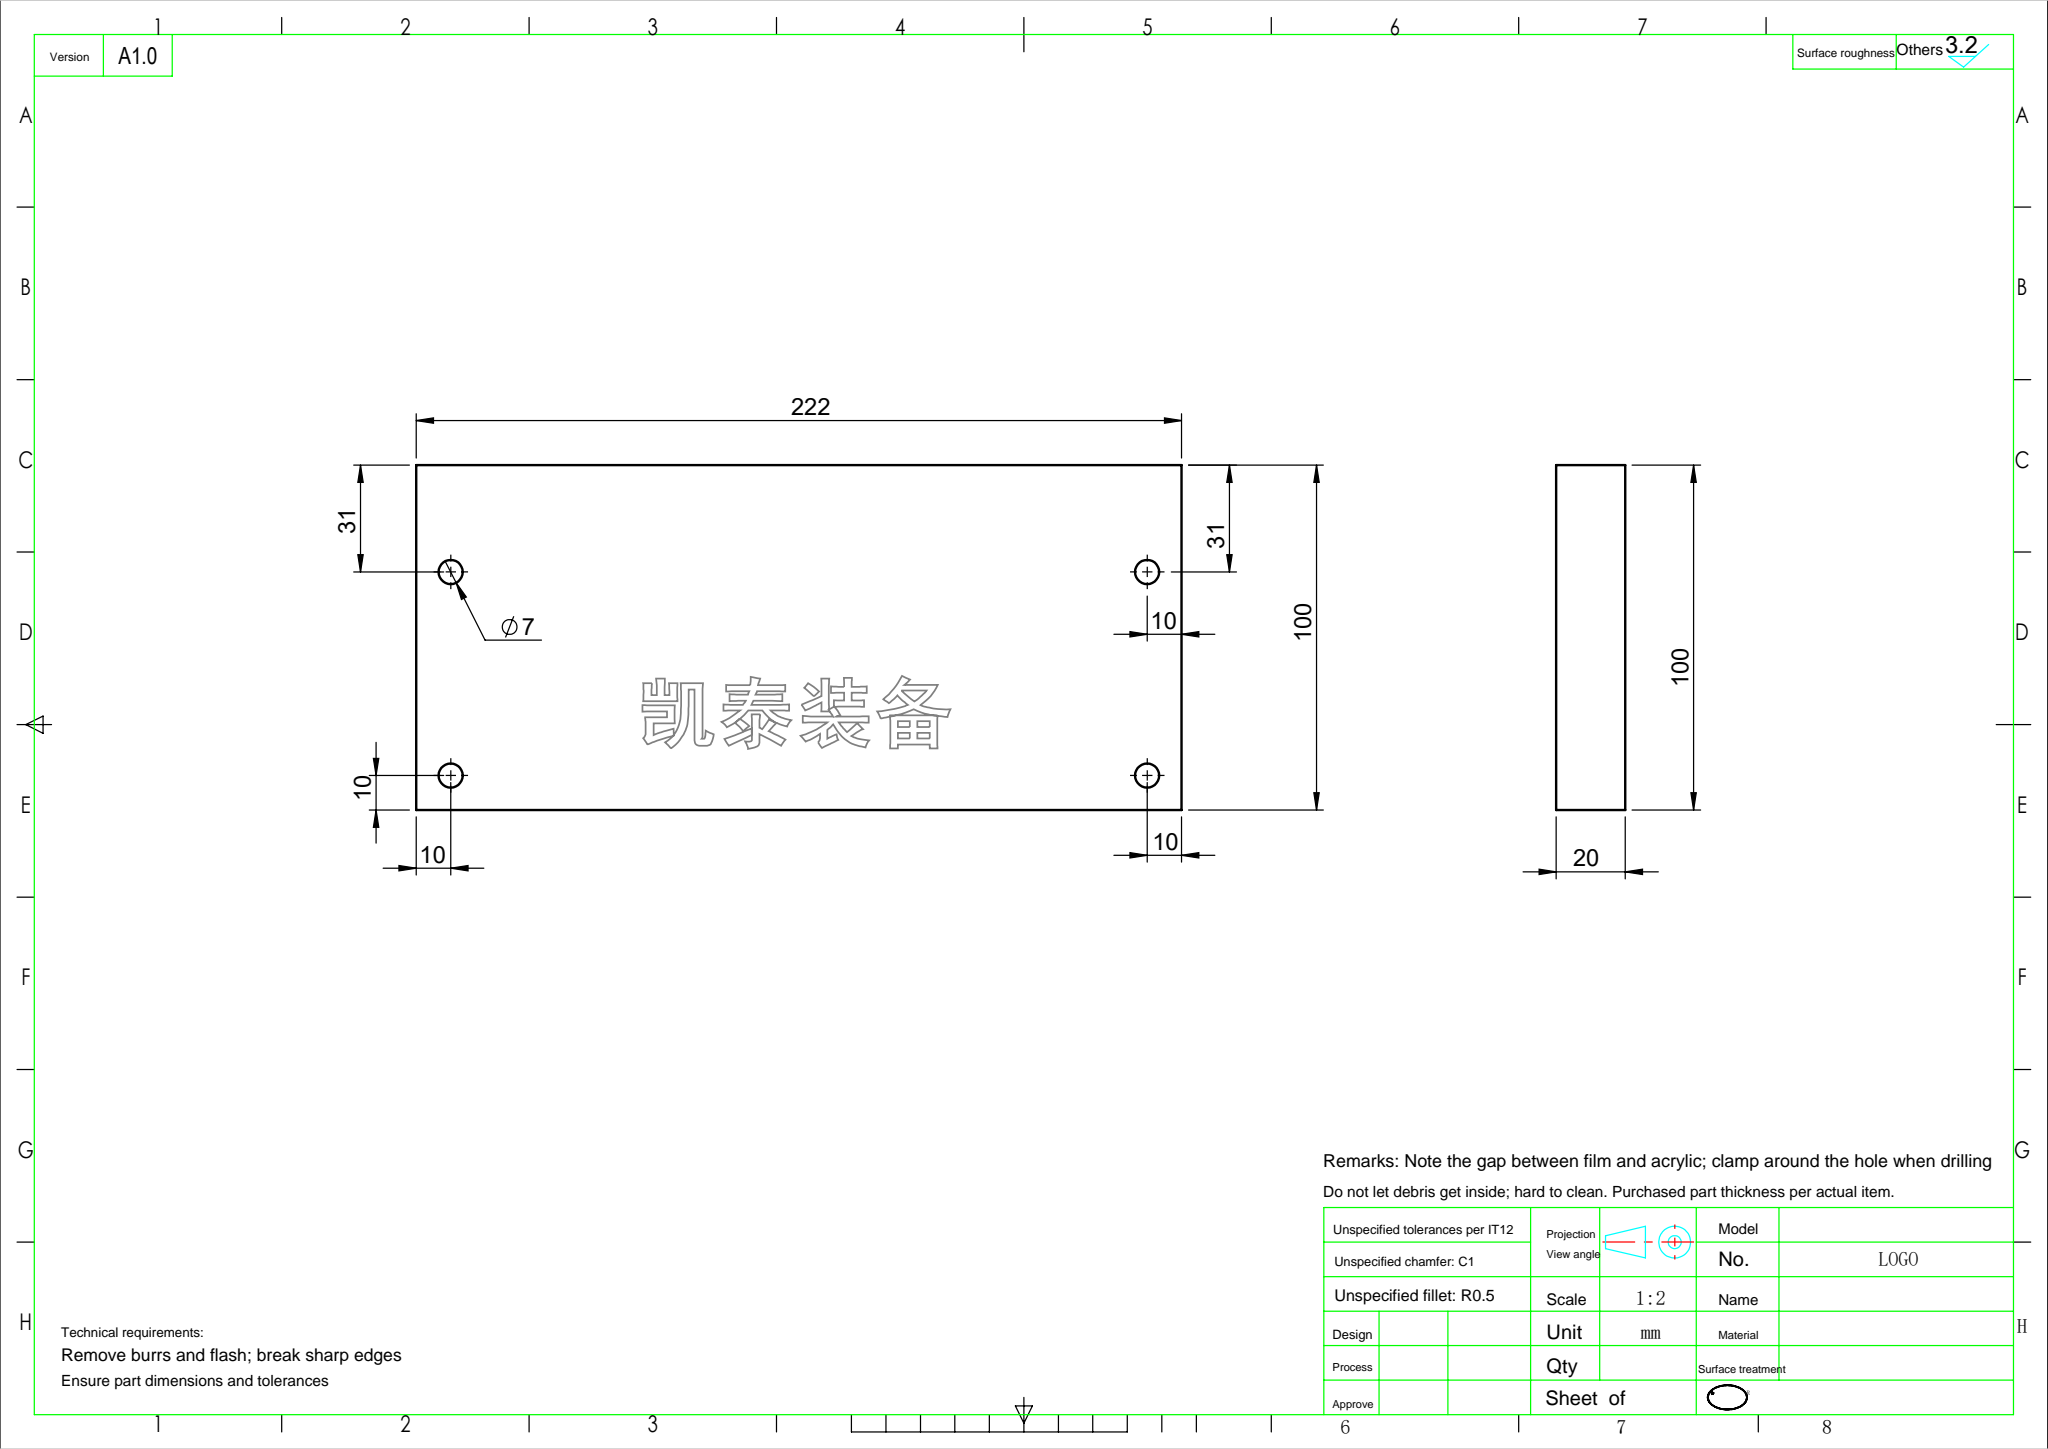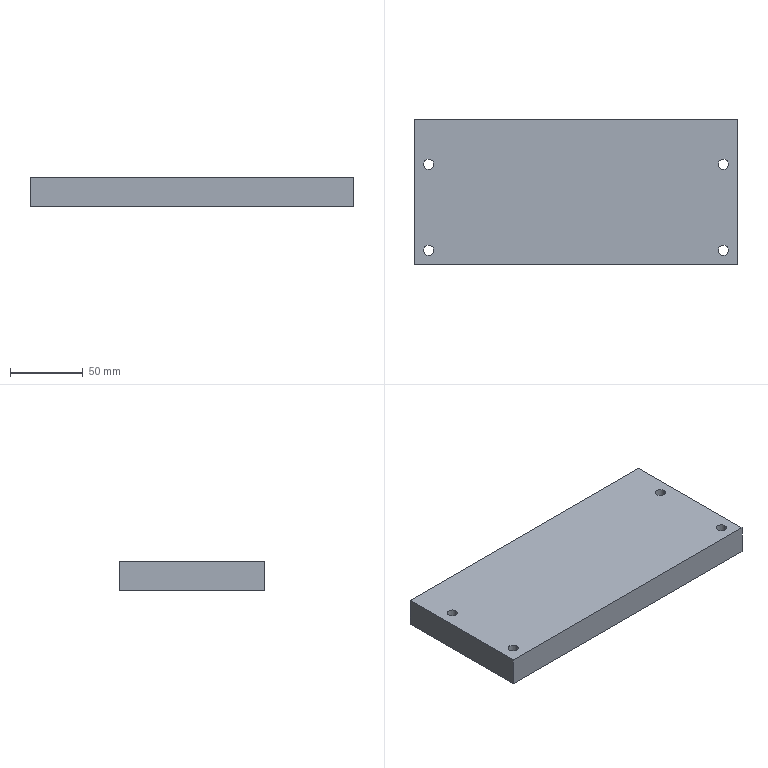Part | SolidWorks | features Extrusion 1, ICE 1 | 1 solid | 14 faces | box 222 x 100 x 20 mm | volume 440921 mm3 | cylinder 8 | plane 6 | commonest cylinder face diameters 7 x8
STEP:
#1=CARTESIAN_POINT('',(-104.5,-40.,0.));
#2=VERTEX_POINT('',#1);
#3=CARTESIAN_POINT('',(-97.5,-40.,0.));
#4=VERTEX_POINT('',#3);
#5=CARTESIAN_POINT('',(-101.,-40.,0.));
#6=DIRECTION('',(0.,0.,1.));
#7=DIRECTION('',(1.,0.,0.));
#8=AXIS2_PLACEMENT_3D('',#5,#6,#7);
#9=CIRCLE('',#8,3.5);
#10=EDGE_CURVE('',#2,#4,#9,.T.);
#11=ORIENTED_EDGE('',*,*,#10,.F.);
#12=CARTESIAN_POINT('',(-104.5,-40.,20.));
#13=VERTEX_POINT('',#12);
#14=CARTESIAN_POINT('',(-104.5,-40.,0.));
#15=DIRECTION('',(0.,0.,1.));
#16=VECTOR('',#15,1000.);
#17=LINE('',#14,#16);
#18=EDGE_CURVE('',#2,#13,#17,.T.);
#19=ORIENTED_EDGE('',*,*,#18,.T.);
#20=CARTESIAN_POINT('',(-97.5,-40.,20.));
#21=VERTEX_POINT('',#20);
#22=CARTESIAN_POINT('',(-101.,-40.,20.));
#23=DIRECTION('',(0.,0.,1.));
#24=DIRECTION('',(1.,0.,0.));
#25=AXIS2_PLACEMENT_3D('',#22,#23,#24);
#26=CIRCLE('',#25,3.5);
#27=EDGE_CURVE('',#13,#21,#26,.T.);
#28=ORIENTED_EDGE('',*,*,#27,.T.);
#29=CARTESIAN_POINT('',(-97.5,-40.,0.));
#30=DIRECTION('',(0.,0.,1.));
#31=VECTOR('',#30,1000.);
#32=LINE('',#29,#31);
#33=EDGE_CURVE('',#4,#21,#32,.T.);
#34=ORIENTED_EDGE('',*,*,#33,.F.);
#35=EDGE_LOOP('',(#11,#19,#28,#34));
#36=FACE_OUTER_BOUND('',#35,.T.);
#37=CARTESIAN_POINT('',(-101.,-40.,0.));
#38=DIRECTION('',(0.,0.,1.));
#39=DIRECTION('',(1.,0.,0.));
#40=AXIS2_PLACEMENT_3D('',#37,#38,#39);
#41=CYLINDRICAL_SURFACE('',#40,3.5);
#42=ADVANCED_FACE('',(#36),#41,.F.);
#43=CARTESIAN_POINT('',(97.5,19.,0.));
#44=VERTEX_POINT('',#43);
#45=CARTESIAN_POINT('',(104.5,19.,0.));
#46=VERTEX_POINT('',#45);
#47=CARTESIAN_POINT('',(101.,19.,0.));
#48=DIRECTION('',(0.,0.,1.));
#49=DIRECTION('',(1.,0.,0.));
#50=AXIS2_PLACEMENT_3D('',#47,#48,#49);
#51=CIRCLE('',#50,3.5);
#52=EDGE_CURVE('',#44,#46,#51,.T.);
#53=ORIENTED_EDGE('',*,*,#52,.F.);
#54=CARTESIAN_POINT('',(97.5,19.,20.));
#55=VERTEX_POINT('',#54);
#56=CARTESIAN_POINT('',(97.5,19.,0.));
#57=DIRECTION('',(0.,0.,1.));
#58=VECTOR('',#57,1000.);
#59=LINE('',#56,#58);
#60=EDGE_CURVE('',#44,#55,#59,.T.);
#61=ORIENTED_EDGE('',*,*,#60,.T.);
#62=CARTESIAN_POINT('',(104.5,19.,20.));
#63=VERTEX_POINT('',#62);
#64=CARTESIAN_POINT('',(101.,19.,20.));
#65=DIRECTION('',(0.,0.,1.));
#66=DIRECTION('',(1.,0.,0.));
#67=AXIS2_PLACEMENT_3D('',#64,#65,#66);
#68=CIRCLE('',#67,3.5);
#69=EDGE_CURVE('',#55,#63,#68,.T.);
#70=ORIENTED_EDGE('',*,*,#69,.T.);
#71=CARTESIAN_POINT('',(104.5,19.,0.));
#72=DIRECTION('',(0.,0.,1.));
#73=VECTOR('',#72,1000.);
#74=LINE('',#71,#73);
#75=EDGE_CURVE('',#46,#63,#74,.T.);
#76=ORIENTED_EDGE('',*,*,#75,.F.);
#77=EDGE_LOOP('',(#53,#61,#70,#76));
#78=FACE_OUTER_BOUND('',#77,.T.);
#79=CARTESIAN_POINT('',(101.,19.,0.));
#80=DIRECTION('',(0.,0.,1.));
#81=DIRECTION('',(1.,0.,0.));
#82=AXIS2_PLACEMENT_3D('',#79,#80,#81);
#83=CYLINDRICAL_SURFACE('',#82,3.5);
#84=ADVANCED_FACE('',(#78),#83,.F.);
#85=CARTESIAN_POINT('',(97.5,-40.,0.));
#86=VERTEX_POINT('',#85);
#87=CARTESIAN_POINT('',(104.5,-40.,0.));
#88=VERTEX_POINT('',#87);
#89=CARTESIAN_POINT('',(101.,-40.,0.));
#90=DIRECTION('',(0.,0.,1.));
#91=DIRECTION('',(1.,0.,0.));
#92=AXIS2_PLACEMENT_3D('',#89,#90,#91);
#93=CIRCLE('',#92,3.5);
#94=EDGE_CURVE('',#86,#88,#93,.T.);
#95=ORIENTED_EDGE('',*,*,#94,.F.);
#96=CARTESIAN_POINT('',(97.5,-40.,20.));
#97=VERTEX_POINT('',#96);
#98=CARTESIAN_POINT('',(97.5,-40.,0.));
#99=DIRECTION('',(0.,0.,1.));
#100=VECTOR('',#99,1000.);
#101=LINE('',#98,#100);
#102=EDGE_CURVE('',#86,#97,#101,.T.);
#103=ORIENTED_EDGE('',*,*,#102,.T.);
#104=CARTESIAN_POINT('',(104.5,-40.,20.));
#105=VERTEX_POINT('',#104);
#106=CARTESIAN_POINT('',(101.,-40.,20.));
#107=DIRECTION('',(0.,0.,1.));
#108=DIRECTION('',(1.,0.,0.));
#109=AXIS2_PLACEMENT_3D('',#106,#107,#108);
#110=CIRCLE('',#109,3.5);
#111=EDGE_CURVE('',#97,#105,#110,.T.);
#112=ORIENTED_EDGE('',*,*,#111,.T.);
#113=CARTESIAN_POINT('',(104.5,-40.,0.));
#114=DIRECTION('',(0.,0.,1.));
#115=VECTOR('',#114,1000.);
#116=LINE('',#113,#115);
#117=EDGE_CURVE('',#88,#105,#116,.T.);
#118=ORIENTED_EDGE('',*,*,#117,.F.);
#119=EDGE_LOOP('',(#95,#103,#112,#118));
#120=FACE_OUTER_BOUND('',#119,.T.);
#121=CARTESIAN_POINT('',(101.,-40.,0.));
#122=DIRECTION('',(0.,0.,1.));
#123=DIRECTION('',(1.,0.,0.));
#124=AXIS2_PLACEMENT_3D('',#121,#122,#123);
#125=CYLINDRICAL_SURFACE('',#124,3.5);
#126=ADVANCED_FACE('',(#120),#125,.F.);
#127=CARTESIAN_POINT('',(-104.5,19.,0.));
#128=VERTEX_POINT('',#127);
#129=CARTESIAN_POINT('',(-97.5,19.,0.));
#130=VERTEX_POINT('',#129);
#131=CARTESIAN_POINT('',(-101.,19.,0.));
#132=DIRECTION('',(0.,0.,1.));
#133=DIRECTION('',(1.,0.,0.));
#134=AXIS2_PLACEMENT_3D('',#131,#132,#133);
#135=CIRCLE('',#134,3.5);
#136=EDGE_CURVE('',#128,#130,#135,.T.);
#137=ORIENTED_EDGE('',*,*,#136,.F.);
#138=CARTESIAN_POINT('',(-104.5,19.,20.));
#139=VERTEX_POINT('',#138);
#140=CARTESIAN_POINT('',(-104.5,19.,0.));
#141=DIRECTION('',(0.,0.,1.));
#142=VECTOR('',#141,1000.);
#143=LINE('',#140,#142);
#144=EDGE_CURVE('',#128,#139,#143,.T.);
#145=ORIENTED_EDGE('',*,*,#144,.T.);
#146=CARTESIAN_POINT('',(-97.5,19.,20.));
#147=VERTEX_POINT('',#146);
#148=CARTESIAN_POINT('',(-101.,19.,20.));
#149=DIRECTION('',(0.,0.,1.));
#150=DIRECTION('',(1.,0.,0.));
#151=AXIS2_PLACEMENT_3D('',#148,#149,#150);
#152=CIRCLE('',#151,3.5);
#153=EDGE_CURVE('',#139,#147,#152,.T.);
#154=ORIENTED_EDGE('',*,*,#153,.T.);
#155=CARTESIAN_POINT('',(-97.5,19.,0.));
#156=DIRECTION('',(0.,0.,1.));
#157=VECTOR('',#156,1000.);
#158=LINE('',#155,#157);
#159=EDGE_CURVE('',#130,#147,#158,.T.);
#160=ORIENTED_EDGE('',*,*,#159,.F.);
#161=EDGE_LOOP('',(#137,#145,#154,#160));
#162=FACE_OUTER_BOUND('',#161,.T.);
#163=CARTESIAN_POINT('',(-101.,19.,0.));
#164=DIRECTION('',(0.,0.,1.));
#165=DIRECTION('',(1.,0.,0.));
#166=AXIS2_PLACEMENT_3D('',#163,#164,#165);
#167=CYLINDRICAL_SURFACE('',#166,3.5);
#168=ADVANCED_FACE('',(#162),#167,.F.);
#169=CARTESIAN_POINT('',(111.,-50.,0.));
#170=VERTEX_POINT('',#169);
#171=CARTESIAN_POINT('',(111.,50.,0.));
#172=VERTEX_POINT('',#171);
#173=CARTESIAN_POINT('',(111.,50.,0.));
#174=DIRECTION('',(0.,1.,0.));
#175=VECTOR('',#174,1000.);
#176=LINE('',#173,#175);
#177=EDGE_CURVE('',#170,#172,#176,.T.);
#178=ORIENTED_EDGE('',*,*,#177,.T.);
#179=CARTESIAN_POINT('',(111.,50.,20.));
#180=VERTEX_POINT('',#179);
#181=CARTESIAN_POINT('',(111.,50.,20.));
#182=DIRECTION('',(0.,0.,-1.));
#183=VECTOR('',#182,1000.);
#184=LINE('',#181,#183);
#185=EDGE_CURVE('',#180,#172,#184,.T.);
#186=ORIENTED_EDGE('',*,*,#185,.F.);
#187=CARTESIAN_POINT('',(111.,-50.,20.));
#188=VERTEX_POINT('',#187);
#189=CARTESIAN_POINT('',(111.,50.,20.));
#190=DIRECTION('',(0.,1.,0.));
#191=VECTOR('',#190,1000.);
#192=LINE('',#189,#191);
#193=EDGE_CURVE('',#188,#180,#192,.T.);
#194=ORIENTED_EDGE('',*,*,#193,.F.);
#195=CARTESIAN_POINT('',(111.,-50.,20.));
#196=DIRECTION('',(0.,0.,-1.));
#197=VECTOR('',#196,1000.);
#198=LINE('',#195,#197);
#199=EDGE_CURVE('',#188,#170,#198,.T.);
#200=ORIENTED_EDGE('',*,*,#199,.T.);
#201=EDGE_LOOP('',(#178,#186,#194,#200));
#202=FACE_OUTER_BOUND('',#201,.T.);
#203=CARTESIAN_POINT('',(111.,50.,20.));
#204=DIRECTION('',(-1.,0.,0.));
#205=DIRECTION('',(0.,-1.,0.));
#206=AXIS2_PLACEMENT_3D('',#203,#204,#205);
#207=PLANE('',#206);
#208=ADVANCED_FACE('',(#202),#207,.F.);
#209=CARTESIAN_POINT('',(-111.,50.,0.));
#210=VERTEX_POINT('',#209);
#211=CARTESIAN_POINT('',(-111.,50.,0.));
#212=DIRECTION('',(-1.,0.,0.));
#213=VECTOR('',#212,1000.);
#214=LINE('',#211,#213);
#215=EDGE_CURVE('',#172,#210,#214,.T.);
#216=ORIENTED_EDGE('',*,*,#215,.T.);
#217=CARTESIAN_POINT('',(-111.,50.,20.));
#218=VERTEX_POINT('',#217);
#219=CARTESIAN_POINT('',(-111.,50.,20.));
#220=DIRECTION('',(0.,0.,-1.));
#221=VECTOR('',#220,1000.);
#222=LINE('',#219,#221);
#223=EDGE_CURVE('',#218,#210,#222,.T.);
#224=ORIENTED_EDGE('',*,*,#223,.F.);
#225=CARTESIAN_POINT('',(-111.,50.,20.));
#226=DIRECTION('',(-1.,0.,0.));
#227=VECTOR('',#226,1000.);
#228=LINE('',#225,#227);
#229=EDGE_CURVE('',#180,#218,#228,.T.);
#230=ORIENTED_EDGE('',*,*,#229,.F.);
#231=ORIENTED_EDGE('',*,*,#185,.T.);
#232=EDGE_LOOP('',(#216,#224,#230,#231));
#233=FACE_OUTER_BOUND('',#232,.T.);
#234=CARTESIAN_POINT('',(-111.,50.,20.));
#235=DIRECTION('',(0.,-1.,0.));
#236=DIRECTION('',(0.,0.,-1.));
#237=AXIS2_PLACEMENT_3D('',#234,#235,#236);
#238=PLANE('',#237);
#239=ADVANCED_FACE('',(#233),#238,.F.);
#240=CARTESIAN_POINT('',(-111.,-50.,0.));
#241=VERTEX_POINT('',#240);
#242=CARTESIAN_POINT('',(-111.,50.,0.));
#243=DIRECTION('',(0.,-1.,0.));
#244=VECTOR('',#243,1000.);
#245=LINE('',#242,#244);
#246=EDGE_CURVE('',#210,#241,#245,.T.);
#247=ORIENTED_EDGE('',*,*,#246,.T.);
#248=CARTESIAN_POINT('',(-111.,-50.,20.));
#249=VERTEX_POINT('',#248);
#250=CARTESIAN_POINT('',(-111.,-50.,20.));
#251=DIRECTION('',(0.,0.,-1.));
#252=VECTOR('',#251,1000.);
#253=LINE('',#250,#252);
#254=EDGE_CURVE('',#249,#241,#253,.T.);
#255=ORIENTED_EDGE('',*,*,#254,.F.);
#256=CARTESIAN_POINT('',(-111.,50.,20.));
#257=DIRECTION('',(0.,-1.,0.));
#258=VECTOR('',#257,1000.);
#259=LINE('',#256,#258);
#260=EDGE_CURVE('',#218,#249,#259,.T.);
#261=ORIENTED_EDGE('',*,*,#260,.F.);
#262=ORIENTED_EDGE('',*,*,#223,.T.);
#263=EDGE_LOOP('',(#247,#255,#261,#262));
#264=FACE_OUTER_BOUND('',#263,.T.);
#265=CARTESIAN_POINT('',(-111.,50.,20.));
#266=DIRECTION('',(1.,0.,0.));
#267=DIRECTION('',(0.,1.,0.));
#268=AXIS2_PLACEMENT_3D('',#265,#266,#267);
#269=PLANE('',#268);
#270=ADVANCED_FACE('',(#264),#269,.F.);
#271=CARTESIAN_POINT('',(-111.,-50.,0.));
#272=DIRECTION('',(1.,0.,0.));
#273=VECTOR('',#272,1000.);
#274=LINE('',#271,#273);
#275=EDGE_CURVE('',#241,#170,#274,.T.);
#276=ORIENTED_EDGE('',*,*,#275,.T.);
#277=ORIENTED_EDGE('',*,*,#199,.F.);
#278=CARTESIAN_POINT('',(-111.,-50.,20.));
#279=DIRECTION('',(1.,0.,0.));
#280=VECTOR('',#279,1000.);
#281=LINE('',#278,#280);
#282=EDGE_CURVE('',#249,#188,#281,.T.);
#283=ORIENTED_EDGE('',*,*,#282,.F.);
#284=ORIENTED_EDGE('',*,*,#254,.T.);
#285=EDGE_LOOP('',(#276,#277,#283,#284));
#286=FACE_OUTER_BOUND('',#285,.T.);
#287=CARTESIAN_POINT('',(-111.,-50.,20.));
#288=DIRECTION('',(0.,1.,0.));
#289=DIRECTION('',(0.,0.,1.));
#290=AXIS2_PLACEMENT_3D('',#287,#288,#289);
#291=PLANE('',#290);
#292=ADVANCED_FACE('',(#286),#291,.F.);
#293=CARTESIAN_POINT('',(-101.,-40.,20.));
#294=DIRECTION('',(0.,0.,1.));
#295=DIRECTION('',(1.,0.,0.));
#296=AXIS2_PLACEMENT_3D('',#293,#294,#295);
#297=CIRCLE('',#296,3.5);
#298=EDGE_CURVE('',#21,#13,#297,.T.);
#299=ORIENTED_EDGE('',*,*,#298,.F.);
#300=ORIENTED_EDGE('',*,*,#27,.F.);
#301=EDGE_LOOP('',(#299,#300));
#302=FACE_BOUND('',#301,.T.);
#303=CARTESIAN_POINT('',(101.,19.,20.));
#304=DIRECTION('',(0.,0.,1.));
#305=DIRECTION('',(1.,0.,0.));
#306=AXIS2_PLACEMENT_3D('',#303,#304,#305);
#307=CIRCLE('',#306,3.5);
#308=EDGE_CURVE('',#63,#55,#307,.T.);
#309=ORIENTED_EDGE('',*,*,#308,.F.);
#310=ORIENTED_EDGE('',*,*,#69,.F.);
#311=EDGE_LOOP('',(#309,#310));
#312=FACE_BOUND('',#311,.T.);
#313=CARTESIAN_POINT('',(101.,-40.,20.));
#314=DIRECTION('',(0.,0.,1.));
#315=DIRECTION('',(1.,0.,0.));
#316=AXIS2_PLACEMENT_3D('',#313,#314,#315);
#317=CIRCLE('',#316,3.5);
#318=EDGE_CURVE('',#105,#97,#317,.T.);
#319=ORIENTED_EDGE('',*,*,#318,.F.);
#320=ORIENTED_EDGE('',*,*,#111,.F.);
#321=EDGE_LOOP('',(#319,#320));
#322=FACE_BOUND('',#321,.T.);
#323=CARTESIAN_POINT('',(-101.,19.,20.));
#324=DIRECTION('',(0.,0.,1.));
#325=DIRECTION('',(1.,0.,0.));
#326=AXIS2_PLACEMENT_3D('',#323,#324,#325);
#327=CIRCLE('',#326,3.5);
#328=EDGE_CURVE('',#147,#139,#327,.T.);
#329=ORIENTED_EDGE('',*,*,#328,.F.);
#330=ORIENTED_EDGE('',*,*,#153,.F.);
#331=EDGE_LOOP('',(#329,#330));
#332=FACE_BOUND('',#331,.T.);
#333=ORIENTED_EDGE('',*,*,#193,.T.);
#334=ORIENTED_EDGE('',*,*,#229,.T.);
#335=ORIENTED_EDGE('',*,*,#260,.T.);
#336=ORIENTED_EDGE('',*,*,#282,.T.);
#337=EDGE_LOOP('',(#333,#334,#335,#336));
#338=FACE_OUTER_BOUND('',#337,.T.);
#339=CARTESIAN_POINT('',(0.,0.,20.));
#340=DIRECTION('',(0.,0.,1.));
#341=DIRECTION('',(1.,0.,0.));
#342=AXIS2_PLACEMENT_3D('',#339,#340,#341);
#343=PLANE('',#342);
#344=ADVANCED_FACE('',(#302,#312,#322,#332,#338),#343,.T.);
#345=CARTESIAN_POINT('',(-101.,-40.,0.));
#346=DIRECTION('',(0.,0.,1.));
#347=DIRECTION('',(1.,0.,0.));
#348=AXIS2_PLACEMENT_3D('',#345,#346,#347);
#349=CIRCLE('',#348,3.5);
#350=EDGE_CURVE('',#4,#2,#349,.T.);
#351=ORIENTED_EDGE('',*,*,#350,.T.);
#352=ORIENTED_EDGE('',*,*,#10,.T.);
#353=EDGE_LOOP('',(#351,#352));
#354=FACE_BOUND('',#353,.T.);
#355=CARTESIAN_POINT('',(101.,19.,0.));
#356=DIRECTION('',(0.,0.,1.));
#357=DIRECTION('',(1.,0.,0.));
#358=AXIS2_PLACEMENT_3D('',#355,#356,#357);
#359=CIRCLE('',#358,3.5);
#360=EDGE_CURVE('',#46,#44,#359,.T.);
#361=ORIENTED_EDGE('',*,*,#360,.T.);
#362=ORIENTED_EDGE('',*,*,#52,.T.);
#363=EDGE_LOOP('',(#361,#362));
#364=FACE_BOUND('',#363,.T.);
#365=CARTESIAN_POINT('',(101.,-40.,0.));
#366=DIRECTION('',(0.,0.,1.));
#367=DIRECTION('',(1.,0.,0.));
#368=AXIS2_PLACEMENT_3D('',#365,#366,#367);
#369=CIRCLE('',#368,3.5);
#370=EDGE_CURVE('',#88,#86,#369,.T.);
#371=ORIENTED_EDGE('',*,*,#370,.T.);
#372=ORIENTED_EDGE('',*,*,#94,.T.);
#373=EDGE_LOOP('',(#371,#372));
#374=FACE_BOUND('',#373,.T.);
#375=CARTESIAN_POINT('',(-101.,19.,0.));
#376=DIRECTION('',(0.,0.,1.));
#377=DIRECTION('',(1.,0.,0.));
#378=AXIS2_PLACEMENT_3D('',#375,#376,#377);
#379=CIRCLE('',#378,3.5);
#380=EDGE_CURVE('',#130,#128,#379,.T.);
#381=ORIENTED_EDGE('',*,*,#380,.T.);
#382=ORIENTED_EDGE('',*,*,#136,.T.);
#383=EDGE_LOOP('',(#381,#382));
#384=FACE_BOUND('',#383,.T.);
#385=ORIENTED_EDGE('',*,*,#177,.F.);
#386=ORIENTED_EDGE('',*,*,#275,.F.);
#387=ORIENTED_EDGE('',*,*,#246,.F.);
#388=ORIENTED_EDGE('',*,*,#215,.F.);
#389=EDGE_LOOP('',(#385,#386,#387,#388));
#390=FACE_OUTER_BOUND('',#389,.T.);
#391=CARTESIAN_POINT('',(0.,0.,0.));
#392=DIRECTION('',(0.,0.,1.));
#393=DIRECTION('',(1.,0.,0.));
#394=AXIS2_PLACEMENT_3D('',#391,#392,#393);
#395=PLANE('',#394);
#396=ADVANCED_FACE('',(#354,#364,#374,#384,#390),#395,.F.);
#397=ORIENTED_EDGE('',*,*,#144,.F.);
#398=ORIENTED_EDGE('',*,*,#380,.F.);
#399=ORIENTED_EDGE('',*,*,#159,.T.);
#400=ORIENTED_EDGE('',*,*,#328,.T.);
#401=EDGE_LOOP('',(#397,#398,#399,#400));
#402=FACE_OUTER_BOUND('',#401,.T.);
#403=CARTESIAN_POINT('',(-101.,19.,0.));
#404=DIRECTION('',(0.,0.,1.));
#405=DIRECTION('',(1.,0.,0.));
#406=AXIS2_PLACEMENT_3D('',#403,#404,#405);
#407=CYLINDRICAL_SURFACE('',#406,3.5);
#408=ADVANCED_FACE('',(#402),#407,.F.);
#409=ORIENTED_EDGE('',*,*,#102,.F.);
#410=ORIENTED_EDGE('',*,*,#370,.F.);
#411=ORIENTED_EDGE('',*,*,#117,.T.);
#412=ORIENTED_EDGE('',*,*,#318,.T.);
#413=EDGE_LOOP('',(#409,#410,#411,#412));
#414=FACE_OUTER_BOUND('',#413,.T.);
#415=CARTESIAN_POINT('',(101.,-40.,0.));
#416=DIRECTION('',(0.,0.,1.));
#417=DIRECTION('',(1.,0.,0.));
#418=AXIS2_PLACEMENT_3D('',#415,#416,#417);
#419=CYLINDRICAL_SURFACE('',#418,3.5);
#420=ADVANCED_FACE('',(#414),#419,.F.);
#421=ORIENTED_EDGE('',*,*,#60,.F.);
#422=ORIENTED_EDGE('',*,*,#360,.F.);
#423=ORIENTED_EDGE('',*,*,#75,.T.);
#424=ORIENTED_EDGE('',*,*,#308,.T.);
#425=EDGE_LOOP('',(#421,#422,#423,#424));
#426=FACE_OUTER_BOUND('',#425,.T.);
#427=CARTESIAN_POINT('',(101.,19.,0.));
#428=DIRECTION('',(0.,0.,1.));
#429=DIRECTION('',(1.,0.,0.));
#430=AXIS2_PLACEMENT_3D('',#427,#428,#429);
#431=CYLINDRICAL_SURFACE('',#430,3.5);
#432=ADVANCED_FACE('',(#426),#431,.F.);
#433=ORIENTED_EDGE('',*,*,#18,.F.);
#434=ORIENTED_EDGE('',*,*,#350,.F.);
#435=ORIENTED_EDGE('',*,*,#33,.T.);
#436=ORIENTED_EDGE('',*,*,#298,.T.);
#437=EDGE_LOOP('',(#433,#434,#435,#436));
#438=FACE_OUTER_BOUND('',#437,.T.);
#439=CARTESIAN_POINT('',(-101.,-40.,0.));
#440=DIRECTION('',(0.,0.,1.));
#441=DIRECTION('',(1.,0.,0.));
#442=AXIS2_PLACEMENT_3D('',#439,#440,#441);
#443=CYLINDRICAL_SURFACE('',#442,3.5);
#444=ADVANCED_FACE('',(#438),#443,.F.);
#445=CLOSED_SHELL('',(#42,#84,#126,#168,#208,#239,#270,#292,#344,#396,#408,#420,#432,#444));
#446=MANIFOLD_SOLID_BREP('',#445);
#447=CARTESIAN_POINT('',(0.,0.,0.));
#448=DIRECTION('',(0.,0.,1.));
#449=DIRECTION('',(1.,0.,0.));
#450=AXIS2_PLACEMENT_3D('',#447,#448,#449);
#451=(LENGTH_UNIT()NAMED_UNIT(*)SI_UNIT(.MILLI.,.METRE.));
#452=UNCERTAINTY_MEASURE_WITH_UNIT(LENGTH_MEASURE(0.00001),#451,'','');
#453=(NAMED_UNIT(*)PLANE_ANGLE_UNIT()SI_UNIT($,.RADIAN.));
#454=(NAMED_UNIT(*)SI_UNIT($,.STERADIAN.)SOLID_ANGLE_UNIT());
#455=(GEOMETRIC_REPRESENTATION_CONTEXT(3)GLOBAL_UNCERTAINTY_ASSIGNED_CONTEXT((#452))GLOBAL_UNIT_ASSIGNED_CONTEXT((#451,#453,#454))REPRESENTATION_CONTEXT('',''));
#456=ADVANCED_BREP_SHAPE_REPRESENTATION('',(#446,#450),#455);